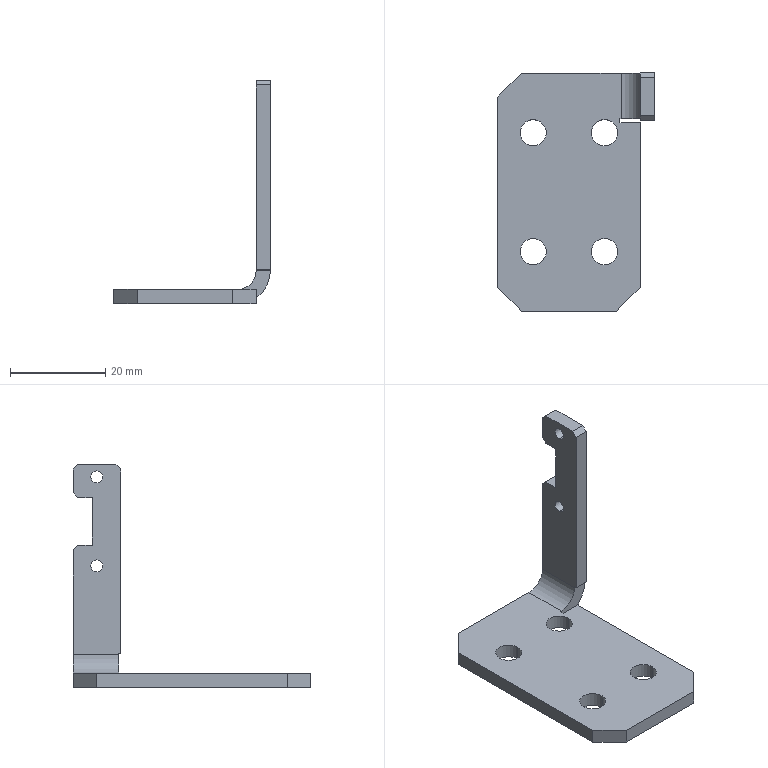Part | STEP file | CON-019 | 1 solid | 43 faces | box 33 x 50 x 47 mm | volume 5269 mm3 | plane 29 | cylinder 14 | commonest cylinder face diameters 5.5 x8 2.5 x4 8 x1 14 x1